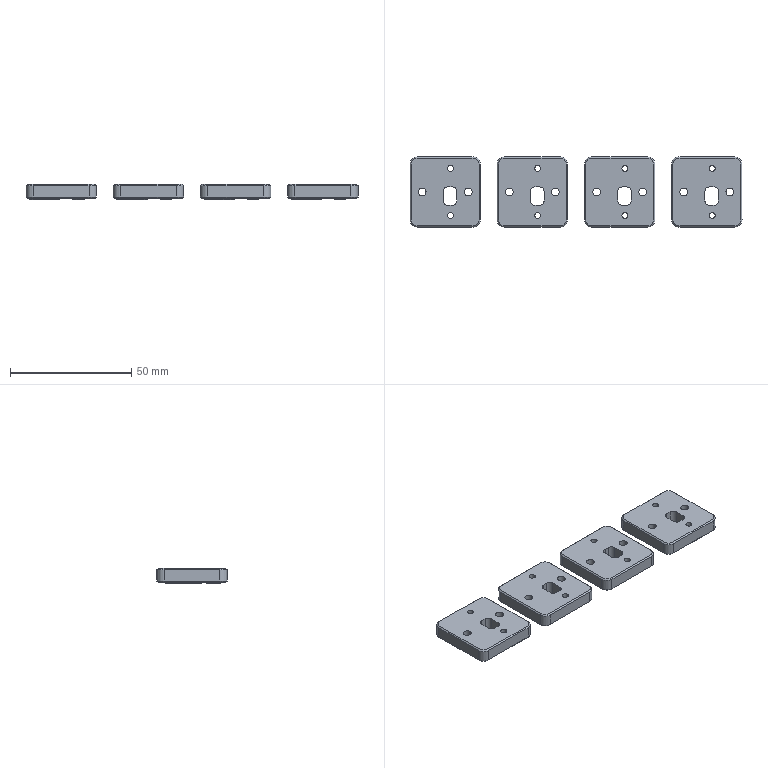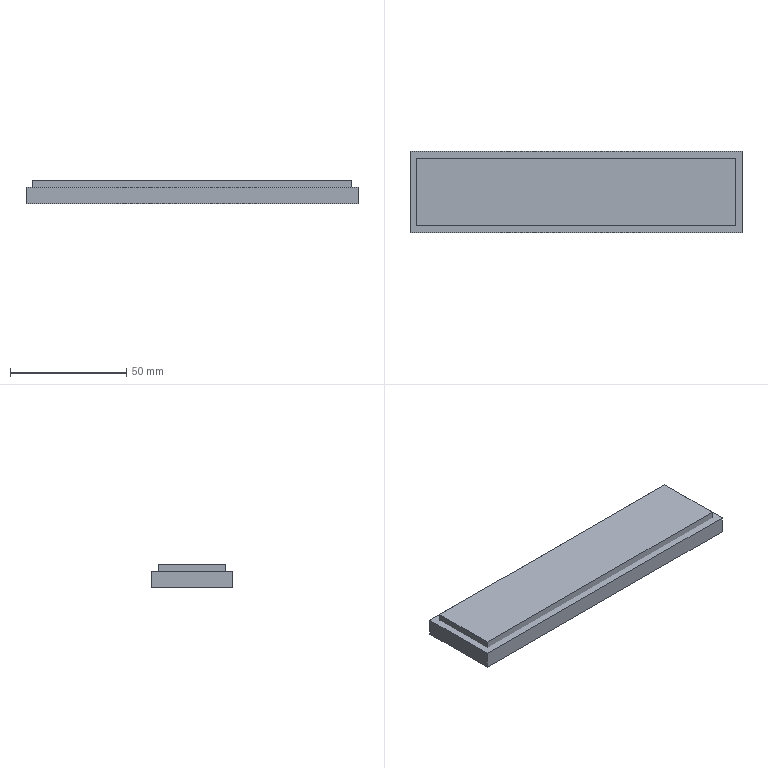CAM job | NX | 3-axis milling, drilling | part box 137 x 29 x 6.3 mm | stock box 143 x 35 x 10.3 mm
Tools:
number,name,description,diameter,corner_radius,flute_length,length,flutes
1,D63,Milling Tool-5 Parameters,63.0,0.0,50.0,75.0,2
2,D4A45,Milling Tool-5 Parameters,4.0,0.0,2.0,2.0,2
13,3.3ZT,Drilling Tool,3.3,0.0,35.0,50.0,2
11,2.5ZT,Drilling Tool,2.5,0.0,35.0,50.0,2
6,D6,Milling Tool-5 Parameters,6.0,0.0,50.0,75.0,2
3,D3,Milling Tool-5 Parameters,3.0,0.0,50.0,75.0,2
12,D2,Milling Tool-5 Parameters,2.0,0.0,50.0,75.0,2
Operations:
program,operation,operation_type,tool,method,geometry_group,spindle_rpm,surface_speed,feed_per_tooth,feed_cut,feed_plunge,cut_length_mm,path_length_mm,cut_time_min,machine_time_min
1虎钳,FLOOR_WALL,VolumeBased25DMillingOperation,D63,METHOD,A,6500.0,1286.0,0.0962,1250.0,100.0,218.0,272.0,0.1744,0.1798
1虎钳,DRILLING_COPY,Operation,D4A45,METHOD,A,5000.0,62.0,0.025,250.0,0.0,57.6,451.232,0.2304,0.2698
1虎钳,DRILLING_COPY_COPY_COPY_COPY_COPY,Operation,2.5ZT,METHOD,A,1910.0,21.0,0.0471,180.0,0.0,87.849,443.594,0.488,0.5236
1虎钳,DRILLING_COPY_COPY_COPY_COPY_COPY_COPY,Operation,3.3ZT,METHOD,A,1910.0,21.0,0.0471,180.0,0.0,92.051,393.832,0.5114,0.5416
1虎钳,ZLEVEL_PROFILE_COPY_COPY_1_COPY,ZLevelMilling,D6,METHOD,A,9500.0,179.0,0.1158,2200.0,1000.0,7045.533,7502.217,3.285,3.331
1虎钳,ZLEVEL_PROFILE_COPY_COPY_COPY_COPY,ZLevelMilling,D6,MILL_FINISH,A,9500.0,119.0,0.0632,1200.0,1000.0,538.435,1031.47,0.4503,0.4996
1虎钳,ZLEVEL_PROFILE_COPY_COPY_1_COPY_COPY,ZLevelMilling,D3,METHOD,A,9500.0,89.0,0.0526,1000.0,1000.0,1953.742,2316.077,1.954,1.99
1虎钳,ZLEVEL_PROFILE_1_COPY_1_COPY_COPY,ZLevelMilling,D4A45,METHOD,A,9500.0,179.0,0.0526,1000.0,100.0,660.027,2675.486,0.66,0.8616
2,FLOOR_WALL_COPY,VolumeBased25DMillingOperation,D63,METHOD,B,6500.0,1286.0,0.0962,1250.0,100.0,848.0,1670.001,0.6784,0.7606
2,FLOOR_WALL_1,VolumeBased25DMillingOperation,D2,METHOD,B,9500.0,59.0,0.0579,1100.0,100.0,14668.018,15090.224,13.335,13.377
2,ZLEVEL_PROFILE_1_COPY_1_COPY_COPY_COPY,ZLevelMilling,D4A45,METHOD,B,9500.0,179.0,0.0526,1000.0,100.0,656.165,2715.821,0.6562,0.8621